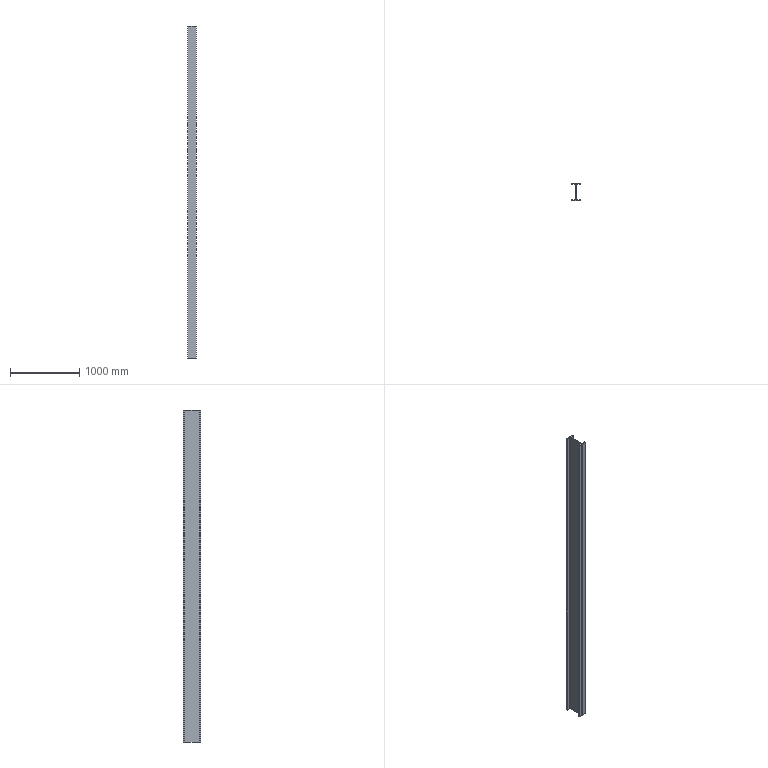Part | SolidWorks | features Extrusion 1 | 1 solid | 18 faces | box 125 x 250 x 4800 mm | volume 17745303 mm3 | plane 14 | cylinder 4 | commonest cylinder face diameters 16 x4
STEP:
#1=CARTESIAN_POINT('',(-62.5,9.,0.));
#2=VERTEX_POINT('',#1);
#3=CARTESIAN_POINT('',(-62.5,0.,0.));
#4=VERTEX_POINT('',#3);
#5=CARTESIAN_POINT('',(-62.5,0.,0.));
#6=DIRECTION('',(0.,-1.,0.));
#7=VECTOR('',#6,1000.);
#8=LINE('',#5,#7);
#9=EDGE_CURVE('',#2,#4,#8,.T.);
#10=ORIENTED_EDGE('',*,*,#9,.T.);
#11=CARTESIAN_POINT('',(-62.5,0.,4800.));
#12=VERTEX_POINT('',#11);
#13=CARTESIAN_POINT('',(-62.5,0.,4800.));
#14=DIRECTION('',(0.,0.,-1.));
#15=VECTOR('',#14,1000.);
#16=LINE('',#13,#15);
#17=EDGE_CURVE('',#12,#4,#16,.T.);
#18=ORIENTED_EDGE('',*,*,#17,.F.);
#19=CARTESIAN_POINT('',(-62.5,9.,4800.));
#20=VERTEX_POINT('',#19);
#21=CARTESIAN_POINT('',(-62.5,0.,4800.));
#22=DIRECTION('',(0.,-1.,0.));
#23=VECTOR('',#22,1000.);
#24=LINE('',#21,#23);
#25=EDGE_CURVE('',#20,#12,#24,.T.);
#26=ORIENTED_EDGE('',*,*,#25,.F.);
#27=CARTESIAN_POINT('',(-62.5,9.,4800.));
#28=DIRECTION('',(0.,0.,-1.));
#29=VECTOR('',#28,1000.);
#30=LINE('',#27,#29);
#31=EDGE_CURVE('',#20,#2,#30,.T.);
#32=ORIENTED_EDGE('',*,*,#31,.T.);
#33=EDGE_LOOP('',(#10,#18,#26,#32));
#34=FACE_OUTER_BOUND('',#33,.T.);
#35=CARTESIAN_POINT('',(-62.5,0.,4800.));
#36=DIRECTION('',(1.,0.,0.));
#37=DIRECTION('',(0.,0.,-1.));
#38=AXIS2_PLACEMENT_3D('',#35,#36,#37);
#39=PLANE('',#38);
#40=ADVANCED_FACE('',(#34),#39,.F.);
#41=CARTESIAN_POINT('',(62.5,0.,0.));
#42=VERTEX_POINT('',#41);
#43=CARTESIAN_POINT('',(62.5,0.,0.));
#44=DIRECTION('',(1.,0.,0.));
#45=VECTOR('',#44,1000.);
#46=LINE('',#43,#45);
#47=EDGE_CURVE('',#4,#42,#46,.T.);
#48=ORIENTED_EDGE('',*,*,#47,.T.);
#49=CARTESIAN_POINT('',(62.5,0.,4800.));
#50=VERTEX_POINT('',#49);
#51=CARTESIAN_POINT('',(62.5,0.,4800.));
#52=DIRECTION('',(0.,0.,-1.));
#53=VECTOR('',#52,1000.);
#54=LINE('',#51,#53);
#55=EDGE_CURVE('',#50,#42,#54,.T.);
#56=ORIENTED_EDGE('',*,*,#55,.F.);
#57=CARTESIAN_POINT('',(62.5,0.,4800.));
#58=DIRECTION('',(1.,0.,0.));
#59=VECTOR('',#58,1000.);
#60=LINE('',#57,#59);
#61=EDGE_CURVE('',#12,#50,#60,.T.);
#62=ORIENTED_EDGE('',*,*,#61,.F.);
#63=ORIENTED_EDGE('',*,*,#17,.T.);
#64=EDGE_LOOP('',(#48,#56,#62,#63));
#65=FACE_OUTER_BOUND('',#64,.T.);
#66=CARTESIAN_POINT('',(62.5,0.,4800.));
#67=DIRECTION('',(0.,1.,0.));
#68=DIRECTION('',(0.,0.,1.));
#69=AXIS2_PLACEMENT_3D('',#66,#67,#68);
#70=PLANE('',#69);
#71=ADVANCED_FACE('',(#65),#70,.F.);
#72=CARTESIAN_POINT('',(62.5,9.,0.));
#73=VERTEX_POINT('',#72);
#74=CARTESIAN_POINT('',(62.5,0.,0.));
#75=DIRECTION('',(0.,1.,0.));
#76=VECTOR('',#75,1000.);
#77=LINE('',#74,#76);
#78=EDGE_CURVE('',#42,#73,#77,.T.);
#79=ORIENTED_EDGE('',*,*,#78,.T.);
#80=CARTESIAN_POINT('',(62.5,9.,4800.));
#81=VERTEX_POINT('',#80);
#82=CARTESIAN_POINT('',(62.5,9.,4800.));
#83=DIRECTION('',(0.,0.,-1.));
#84=VECTOR('',#83,1000.);
#85=LINE('',#82,#84);
#86=EDGE_CURVE('',#81,#73,#85,.T.);
#87=ORIENTED_EDGE('',*,*,#86,.F.);
#88=CARTESIAN_POINT('',(62.5,0.,4800.));
#89=DIRECTION('',(0.,1.,0.));
#90=VECTOR('',#89,1000.);
#91=LINE('',#88,#90);
#92=EDGE_CURVE('',#50,#81,#91,.T.);
#93=ORIENTED_EDGE('',*,*,#92,.F.);
#94=ORIENTED_EDGE('',*,*,#55,.T.);
#95=EDGE_LOOP('',(#79,#87,#93,#94));
#96=FACE_OUTER_BOUND('',#95,.T.);
#97=CARTESIAN_POINT('',(62.5,0.,4800.));
#98=DIRECTION('',(-1.,0.,0.));
#99=DIRECTION('',(0.,0.,1.));
#100=AXIS2_PLACEMENT_3D('',#97,#98,#99);
#101=PLANE('',#100);
#102=ADVANCED_FACE('',(#96),#101,.F.);
#103=CARTESIAN_POINT('',(11.,9.,0.));
#104=VERTEX_POINT('',#103);
#105=CARTESIAN_POINT('',(62.5,9.,0.));
#106=DIRECTION('',(-1.,0.,0.));
#107=VECTOR('',#106,1000.);
#108=LINE('',#105,#107);
#109=EDGE_CURVE('',#73,#104,#108,.T.);
#110=ORIENTED_EDGE('',*,*,#109,.T.);
#111=CARTESIAN_POINT('',(11.,9.,4800.));
#112=VERTEX_POINT('',#111);
#113=CARTESIAN_POINT('',(11.,9.,4800.));
#114=DIRECTION('',(0.,0.,-1.));
#115=VECTOR('',#114,1000.);
#116=LINE('',#113,#115);
#117=EDGE_CURVE('',#112,#104,#116,.T.);
#118=ORIENTED_EDGE('',*,*,#117,.F.);
#119=CARTESIAN_POINT('',(62.5,9.,4800.));
#120=DIRECTION('',(-1.,0.,0.));
#121=VECTOR('',#120,1000.);
#122=LINE('',#119,#121);
#123=EDGE_CURVE('',#81,#112,#122,.T.);
#124=ORIENTED_EDGE('',*,*,#123,.F.);
#125=ORIENTED_EDGE('',*,*,#86,.T.);
#126=EDGE_LOOP('',(#110,#118,#124,#125));
#127=FACE_OUTER_BOUND('',#126,.T.);
#128=CARTESIAN_POINT('',(62.5,9.,4800.));
#129=DIRECTION('',(0.,-1.,0.));
#130=DIRECTION('',(0.,0.,-1.));
#131=AXIS2_PLACEMENT_3D('',#128,#129,#130);
#132=PLANE('',#131);
#133=ADVANCED_FACE('',(#127),#132,.F.);
#134=CARTESIAN_POINT('',(3.,17.,0.));
#135=VERTEX_POINT('',#134);
#136=CARTESIAN_POINT('',(11.,17.,0.));
#137=DIRECTION('',(0.,0.,-1.));
#138=DIRECTION('',(-1.,0.,0.));
#139=AXIS2_PLACEMENT_3D('',#136,#137,#138);
#140=CIRCLE('',#139,8.);
#141=EDGE_CURVE('',#104,#135,#140,.T.);
#142=ORIENTED_EDGE('',*,*,#141,.T.);
#143=CARTESIAN_POINT('',(3.,17.,4800.));
#144=VERTEX_POINT('',#143);
#145=CARTESIAN_POINT('',(3.,17.,4800.));
#146=DIRECTION('',(0.,0.,-1.));
#147=VECTOR('',#146,1000.);
#148=LINE('',#145,#147);
#149=EDGE_CURVE('',#144,#135,#148,.T.);
#150=ORIENTED_EDGE('',*,*,#149,.F.);
#151=CARTESIAN_POINT('',(11.,17.,4800.));
#152=DIRECTION('',(0.,0.,-1.));
#153=DIRECTION('',(-1.,0.,0.));
#154=AXIS2_PLACEMENT_3D('',#151,#152,#153);
#155=CIRCLE('',#154,8.);
#156=EDGE_CURVE('',#112,#144,#155,.T.);
#157=ORIENTED_EDGE('',*,*,#156,.F.);
#158=ORIENTED_EDGE('',*,*,#117,.T.);
#159=EDGE_LOOP('',(#142,#150,#157,#158));
#160=FACE_OUTER_BOUND('',#159,.T.);
#161=CARTESIAN_POINT('',(11.,17.,4800.));
#162=DIRECTION('',(0.,0.,-1.));
#163=DIRECTION('',(-1.,0.,0.));
#164=AXIS2_PLACEMENT_3D('',#161,#162,#163);
#165=CYLINDRICAL_SURFACE('',#164,8.);
#166=ADVANCED_FACE('',(#160),#165,.F.);
#167=CARTESIAN_POINT('',(3.,233.,0.));
#168=VERTEX_POINT('',#167);
#169=CARTESIAN_POINT('',(3.,17.,0.));
#170=DIRECTION('',(0.,1.,0.));
#171=VECTOR('',#170,1000.);
#172=LINE('',#169,#171);
#173=EDGE_CURVE('',#135,#168,#172,.T.);
#174=ORIENTED_EDGE('',*,*,#173,.T.);
#175=CARTESIAN_POINT('',(3.,233.,4800.));
#176=VERTEX_POINT('',#175);
#177=CARTESIAN_POINT('',(3.,233.,4800.));
#178=DIRECTION('',(0.,0.,-1.));
#179=VECTOR('',#178,1000.);
#180=LINE('',#177,#179);
#181=EDGE_CURVE('',#176,#168,#180,.T.);
#182=ORIENTED_EDGE('',*,*,#181,.F.);
#183=CARTESIAN_POINT('',(3.,17.,4800.));
#184=DIRECTION('',(0.,1.,0.));
#185=VECTOR('',#184,1000.);
#186=LINE('',#183,#185);
#187=EDGE_CURVE('',#144,#176,#186,.T.);
#188=ORIENTED_EDGE('',*,*,#187,.F.);
#189=ORIENTED_EDGE('',*,*,#149,.T.);
#190=EDGE_LOOP('',(#174,#182,#188,#189));
#191=FACE_OUTER_BOUND('',#190,.T.);
#192=CARTESIAN_POINT('',(3.,17.,4800.));
#193=DIRECTION('',(-1.,0.,0.));
#194=DIRECTION('',(0.,-1.,0.));
#195=AXIS2_PLACEMENT_3D('',#192,#193,#194);
#196=PLANE('',#195);
#197=ADVANCED_FACE('',(#191),#196,.F.);
#198=CARTESIAN_POINT('',(11.,241.,0.));
#199=VERTEX_POINT('',#198);
#200=CARTESIAN_POINT('',(11.,233.,0.));
#201=DIRECTION('',(0.,0.,-1.));
#202=DIRECTION('',(-1.,0.,0.));
#203=AXIS2_PLACEMENT_3D('',#200,#201,#202);
#204=CIRCLE('',#203,8.);
#205=EDGE_CURVE('',#168,#199,#204,.T.);
#206=ORIENTED_EDGE('',*,*,#205,.T.);
#207=CARTESIAN_POINT('',(11.,241.,4800.));
#208=VERTEX_POINT('',#207);
#209=CARTESIAN_POINT('',(11.,241.,4800.));
#210=DIRECTION('',(0.,0.,-1.));
#211=VECTOR('',#210,1000.);
#212=LINE('',#209,#211);
#213=EDGE_CURVE('',#208,#199,#212,.T.);
#214=ORIENTED_EDGE('',*,*,#213,.F.);
#215=CARTESIAN_POINT('',(11.,233.,4800.));
#216=DIRECTION('',(0.,0.,-1.));
#217=DIRECTION('',(-1.,0.,0.));
#218=AXIS2_PLACEMENT_3D('',#215,#216,#217);
#219=CIRCLE('',#218,8.);
#220=EDGE_CURVE('',#176,#208,#219,.T.);
#221=ORIENTED_EDGE('',*,*,#220,.F.);
#222=ORIENTED_EDGE('',*,*,#181,.T.);
#223=EDGE_LOOP('',(#206,#214,#221,#222));
#224=FACE_OUTER_BOUND('',#223,.T.);
#225=CARTESIAN_POINT('',(11.,233.,4800.));
#226=DIRECTION('',(0.,0.,-1.));
#227=DIRECTION('',(-1.,0.,0.));
#228=AXIS2_PLACEMENT_3D('',#225,#226,#227);
#229=CYLINDRICAL_SURFACE('',#228,8.);
#230=ADVANCED_FACE('',(#224),#229,.F.);
#231=CARTESIAN_POINT('',(62.5,241.,0.));
#232=VERTEX_POINT('',#231);
#233=CARTESIAN_POINT('',(11.,241.,0.));
#234=DIRECTION('',(1.,0.,0.));
#235=VECTOR('',#234,1000.);
#236=LINE('',#233,#235);
#237=EDGE_CURVE('',#199,#232,#236,.T.);
#238=ORIENTED_EDGE('',*,*,#237,.T.);
#239=CARTESIAN_POINT('',(62.5,241.,4800.));
#240=VERTEX_POINT('',#239);
#241=CARTESIAN_POINT('',(62.5,241.,4800.));
#242=DIRECTION('',(0.,0.,-1.));
#243=VECTOR('',#242,1000.);
#244=LINE('',#241,#243);
#245=EDGE_CURVE('',#240,#232,#244,.T.);
#246=ORIENTED_EDGE('',*,*,#245,.F.);
#247=CARTESIAN_POINT('',(11.,241.,4800.));
#248=DIRECTION('',(1.,0.,0.));
#249=VECTOR('',#248,1000.);
#250=LINE('',#247,#249);
#251=EDGE_CURVE('',#208,#240,#250,.T.);
#252=ORIENTED_EDGE('',*,*,#251,.F.);
#253=ORIENTED_EDGE('',*,*,#213,.T.);
#254=EDGE_LOOP('',(#238,#246,#252,#253));
#255=FACE_OUTER_BOUND('',#254,.T.);
#256=CARTESIAN_POINT('',(11.,241.,4800.));
#257=DIRECTION('',(0.,1.,0.));
#258=DIRECTION('',(0.,0.,1.));
#259=AXIS2_PLACEMENT_3D('',#256,#257,#258);
#260=PLANE('',#259);
#261=ADVANCED_FACE('',(#255),#260,.F.);
#262=CARTESIAN_POINT('',(62.5,250.,0.));
#263=VERTEX_POINT('',#262);
#264=CARTESIAN_POINT('',(62.5,241.,0.));
#265=DIRECTION('',(0.,1.,0.));
#266=VECTOR('',#265,1000.);
#267=LINE('',#264,#266);
#268=EDGE_CURVE('',#232,#263,#267,.T.);
#269=ORIENTED_EDGE('',*,*,#268,.T.);
#270=CARTESIAN_POINT('',(62.5,250.,4800.));
#271=VERTEX_POINT('',#270);
#272=CARTESIAN_POINT('',(62.5,250.,4800.));
#273=DIRECTION('',(0.,0.,-1.));
#274=VECTOR('',#273,1000.);
#275=LINE('',#272,#274);
#276=EDGE_CURVE('',#271,#263,#275,.T.);
#277=ORIENTED_EDGE('',*,*,#276,.F.);
#278=CARTESIAN_POINT('',(62.5,241.,4800.));
#279=DIRECTION('',(0.,1.,0.));
#280=VECTOR('',#279,1000.);
#281=LINE('',#278,#280);
#282=EDGE_CURVE('',#240,#271,#281,.T.);
#283=ORIENTED_EDGE('',*,*,#282,.F.);
#284=ORIENTED_EDGE('',*,*,#245,.T.);
#285=EDGE_LOOP('',(#269,#277,#283,#284));
#286=FACE_OUTER_BOUND('',#285,.T.);
#287=CARTESIAN_POINT('',(62.5,241.,4800.));
#288=DIRECTION('',(-1.,0.,0.));
#289=DIRECTION('',(0.,0.,1.));
#290=AXIS2_PLACEMENT_3D('',#287,#288,#289);
#291=PLANE('',#290);
#292=ADVANCED_FACE('',(#286),#291,.F.);
#293=CARTESIAN_POINT('',(-62.5,250.,0.));
#294=VERTEX_POINT('',#293);
#295=CARTESIAN_POINT('',(-62.5,250.,0.));
#296=DIRECTION('',(-1.,0.,0.));
#297=VECTOR('',#296,1000.);
#298=LINE('',#295,#297);
#299=EDGE_CURVE('',#263,#294,#298,.T.);
#300=ORIENTED_EDGE('',*,*,#299,.T.);
#301=CARTESIAN_POINT('',(-62.5,250.,4800.));
#302=VERTEX_POINT('',#301);
#303=CARTESIAN_POINT('',(-62.5,250.,4800.));
#304=DIRECTION('',(0.,0.,-1.));
#305=VECTOR('',#304,1000.);
#306=LINE('',#303,#305);
#307=EDGE_CURVE('',#302,#294,#306,.T.);
#308=ORIENTED_EDGE('',*,*,#307,.F.);
#309=CARTESIAN_POINT('',(-62.5,250.,4800.));
#310=DIRECTION('',(-1.,0.,0.));
#311=VECTOR('',#310,1000.);
#312=LINE('',#309,#311);
#313=EDGE_CURVE('',#271,#302,#312,.T.);
#314=ORIENTED_EDGE('',*,*,#313,.F.);
#315=ORIENTED_EDGE('',*,*,#276,.T.);
#316=EDGE_LOOP('',(#300,#308,#314,#315));
#317=FACE_OUTER_BOUND('',#316,.T.);
#318=CARTESIAN_POINT('',(-62.5,250.,4800.));
#319=DIRECTION('',(0.,-1.,0.));
#320=DIRECTION('',(1.,0.,0.));
#321=AXIS2_PLACEMENT_3D('',#318,#319,#320);
#322=PLANE('',#321);
#323=ADVANCED_FACE('',(#317),#322,.F.);
#324=CARTESIAN_POINT('',(-62.5,241.,0.));
#325=VERTEX_POINT('',#324);
#326=CARTESIAN_POINT('',(-62.5,241.,0.));
#327=DIRECTION('',(0.,-1.,0.));
#328=VECTOR('',#327,1000.);
#329=LINE('',#326,#328);
#330=EDGE_CURVE('',#294,#325,#329,.T.);
#331=ORIENTED_EDGE('',*,*,#330,.T.);
#332=CARTESIAN_POINT('',(-62.5,241.,4800.));
#333=VERTEX_POINT('',#332);
#334=CARTESIAN_POINT('',(-62.5,241.,4800.));
#335=DIRECTION('',(0.,0.,-1.));
#336=VECTOR('',#335,1000.);
#337=LINE('',#334,#336);
#338=EDGE_CURVE('',#333,#325,#337,.T.);
#339=ORIENTED_EDGE('',*,*,#338,.F.);
#340=CARTESIAN_POINT('',(-62.5,241.,4800.));
#341=DIRECTION('',(0.,-1.,0.));
#342=VECTOR('',#341,1000.);
#343=LINE('',#340,#342);
#344=EDGE_CURVE('',#302,#333,#343,.T.);
#345=ORIENTED_EDGE('',*,*,#344,.F.);
#346=ORIENTED_EDGE('',*,*,#307,.T.);
#347=EDGE_LOOP('',(#331,#339,#345,#346));
#348=FACE_OUTER_BOUND('',#347,.T.);
#349=CARTESIAN_POINT('',(-62.5,241.,4800.));
#350=DIRECTION('',(1.,0.,0.));
#351=DIRECTION('',(0.,0.,-1.));
#352=AXIS2_PLACEMENT_3D('',#349,#350,#351);
#353=PLANE('',#352);
#354=ADVANCED_FACE('',(#348),#353,.F.);
#355=CARTESIAN_POINT('',(-11.,241.,0.));
#356=VERTEX_POINT('',#355);
#357=CARTESIAN_POINT('',(-11.,241.,0.));
#358=DIRECTION('',(1.,0.,0.));
#359=VECTOR('',#358,1000.);
#360=LINE('',#357,#359);
#361=EDGE_CURVE('',#325,#356,#360,.T.);
#362=ORIENTED_EDGE('',*,*,#361,.T.);
#363=CARTESIAN_POINT('',(-11.,241.,4800.));
#364=VERTEX_POINT('',#363);
#365=CARTESIAN_POINT('',(-11.,241.,4800.));
#366=DIRECTION('',(0.,0.,-1.));
#367=VECTOR('',#366,1000.);
#368=LINE('',#365,#367);
#369=EDGE_CURVE('',#364,#356,#368,.T.);
#370=ORIENTED_EDGE('',*,*,#369,.F.);
#371=CARTESIAN_POINT('',(-11.,241.,4800.));
#372=DIRECTION('',(1.,0.,0.));
#373=VECTOR('',#372,1000.);
#374=LINE('',#371,#373);
#375=EDGE_CURVE('',#333,#364,#374,.T.);
#376=ORIENTED_EDGE('',*,*,#375,.F.);
#377=ORIENTED_EDGE('',*,*,#338,.T.);
#378=EDGE_LOOP('',(#362,#370,#376,#377));
#379=FACE_OUTER_BOUND('',#378,.T.);
#380=CARTESIAN_POINT('',(-11.,241.,4800.));
#381=DIRECTION('',(0.,1.,0.));
#382=DIRECTION('',(0.,0.,1.));
#383=AXIS2_PLACEMENT_3D('',#380,#381,#382);
#384=PLANE('',#383);
#385=ADVANCED_FACE('',(#379),#384,.F.);
#386=CARTESIAN_POINT('',(-3.,233.,0.));
#387=VERTEX_POINT('',#386);
#388=CARTESIAN_POINT('',(-11.,233.,0.));
#389=DIRECTION('',(0.,0.,-1.));
#390=DIRECTION('',(1.,0.,0.));
#391=AXIS2_PLACEMENT_3D('',#388,#389,#390);
#392=CIRCLE('',#391,8.);
#393=EDGE_CURVE('',#356,#387,#392,.T.);
#394=ORIENTED_EDGE('',*,*,#393,.T.);
#395=CARTESIAN_POINT('',(-3.,233.,4800.));
#396=VERTEX_POINT('',#395);
#397=CARTESIAN_POINT('',(-3.,233.,4800.));
#398=DIRECTION('',(0.,0.,-1.));
#399=VECTOR('',#398,1000.);
#400=LINE('',#397,#399);
#401=EDGE_CURVE('',#396,#387,#400,.T.);
#402=ORIENTED_EDGE('',*,*,#401,.F.);
#403=CARTESIAN_POINT('',(-11.,233.,4800.));
#404=DIRECTION('',(0.,0.,-1.));
#405=DIRECTION('',(1.,0.,0.));
#406=AXIS2_PLACEMENT_3D('',#403,#404,#405);
#407=CIRCLE('',#406,8.);
#408=EDGE_CURVE('',#364,#396,#407,.T.);
#409=ORIENTED_EDGE('',*,*,#408,.F.);
#410=ORIENTED_EDGE('',*,*,#369,.T.);
#411=EDGE_LOOP('',(#394,#402,#409,#410));
#412=FACE_OUTER_BOUND('',#411,.T.);
#413=CARTESIAN_POINT('',(-11.,233.,4800.));
#414=DIRECTION('',(0.,0.,-1.));
#415=DIRECTION('',(-1.,0.,0.));
#416=AXIS2_PLACEMENT_3D('',#413,#414,#415);
#417=CYLINDRICAL_SURFACE('',#416,8.);
#418=ADVANCED_FACE('',(#412),#417,.F.);
#419=CARTESIAN_POINT('',(-3.,17.,0.));
#420=VERTEX_POINT('',#419);
#421=CARTESIAN_POINT('',(-3.,17.,0.));
#422=DIRECTION('',(0.,-1.,0.));
#423=VECTOR('',#422,1000.);
#424=LINE('',#421,#423);
#425=EDGE_CURVE('',#387,#420,#424,.T.);
#426=ORIENTED_EDGE('',*,*,#425,.T.);
#427=CARTESIAN_POINT('',(-3.,17.,4800.));
#428=VERTEX_POINT('',#427);
#429=CARTESIAN_POINT('',(-3.,17.,4800.));
#430=DIRECTION('',(0.,0.,-1.));
#431=VECTOR('',#430,1000.);
#432=LINE('',#429,#431);
#433=EDGE_CURVE('',#428,#420,#432,.T.);
#434=ORIENTED_EDGE('',*,*,#433,.F.);
#435=CARTESIAN_POINT('',(-3.,17.,4800.));
#436=DIRECTION('',(0.,-1.,0.));
#437=VECTOR('',#436,1000.);
#438=LINE('',#435,#437);
#439=EDGE_CURVE('',#396,#428,#438,.T.);
#440=ORIENTED_EDGE('',*,*,#439,.F.);
#441=ORIENTED_EDGE('',*,*,#401,.T.);
#442=EDGE_LOOP('',(#426,#434,#440,#441));
#443=FACE_OUTER_BOUND('',#442,.T.);
#444=CARTESIAN_POINT('',(-3.,17.,4800.));
#445=DIRECTION('',(1.,0.,0.));
#446=DIRECTION('',(0.,1.,0.));
#447=AXIS2_PLACEMENT_3D('',#444,#445,#446);
#448=PLANE('',#447);
#449=ADVANCED_FACE('',(#443),#448,.F.);
#450=CARTESIAN_POINT('',(-11.,9.,0.));
#451=VERTEX_POINT('',#450);
#452=CARTESIAN_POINT('',(-11.,17.,0.));
#453=DIRECTION('',(0.,0.,-1.));
#454=DIRECTION('',(-1.,0.,0.));
#455=AXIS2_PLACEMENT_3D('',#452,#453,#454);
#456=CIRCLE('',#455,8.);
#457=EDGE_CURVE('',#420,#451,#456,.T.);
#458=ORIENTED_EDGE('',*,*,#457,.T.);
#459=CARTESIAN_POINT('',(-11.,9.,4800.));
#460=VERTEX_POINT('',#459);
#461=CARTESIAN_POINT('',(-11.,9.,4800.));
#462=DIRECTION('',(0.,0.,-1.));
#463=VECTOR('',#462,1000.);
#464=LINE('',#461,#463);
#465=EDGE_CURVE('',#460,#451,#464,.T.);
#466=ORIENTED_EDGE('',*,*,#465,.F.);
#467=CARTESIAN_POINT('',(-11.,17.,4800.));
#468=DIRECTION('',(0.,0.,-1.));
#469=DIRECTION('',(-1.,0.,0.));
#470=AXIS2_PLACEMENT_3D('',#467,#468,#469);
#471=CIRCLE('',#470,8.);
#472=EDGE_CURVE('',#428,#460,#471,.T.);
#473=ORIENTED_EDGE('',*,*,#472,.F.);
#474=ORIENTED_EDGE('',*,*,#433,.T.);
#475=EDGE_LOOP('',(#458,#466,#473,#474));
#476=FACE_OUTER_BOUND('',#475,.T.);
#477=CARTESIAN_POINT('',(-11.,17.,4800.));
#478=DIRECTION('',(0.,0.,-1.));
#479=DIRECTION('',(-1.,0.,0.));
#480=AXIS2_PLACEMENT_3D('',#477,#478,#479);
#481=CYLINDRICAL_SURFACE('',#480,8.);
#482=ADVANCED_FACE('',(#476),#481,.F.);
#483=CARTESIAN_POINT('',(-62.5,9.,0.));
#484=DIRECTION('',(-1.,0.,0.));
#485=VECTOR('',#484,1000.);
#486=LINE('',#483,#485);
#487=EDGE_CURVE('',#451,#2,#486,.T.);
#488=ORIENTED_EDGE('',*,*,#487,.T.);
#489=ORIENTED_EDGE('',*,*,#31,.F.);
#490=CARTESIAN_POINT('',(-62.5,9.,4800.));
#491=DIRECTION('',(-1.,0.,0.));
#492=VECTOR('',#491,1000.);
#493=LINE('',#490,#492);
#494=EDGE_CURVE('',#460,#20,#493,.T.);
#495=ORIENTED_EDGE('',*,*,#494,.F.);
#496=ORIENTED_EDGE('',*,*,#465,.T.);
#497=EDGE_LOOP('',(#488,#489,#495,#496));
#498=FACE_OUTER_BOUND('',#497,.T.);
#499=CARTESIAN_POINT('',(-62.5,9.,4800.));
#500=DIRECTION('',(0.,-1.,0.));
#501=DIRECTION('',(0.,0.,-1.));
#502=AXIS2_PLACEMENT_3D('',#499,#500,#501);
#503=PLANE('',#502);
#504=ADVANCED_FACE('',(#498),#503,.F.);
#505=ORIENTED_EDGE('',*,*,#25,.T.);
#506=ORIENTED_EDGE('',*,*,#61,.T.);
#507=ORIENTED_EDGE('',*,*,#92,.T.);
#508=ORIENTED_EDGE('',*,*,#123,.T.);
#509=ORIENTED_EDGE('',*,*,#156,.T.);
#510=ORIENTED_EDGE('',*,*,#187,.T.);
#511=ORIENTED_EDGE('',*,*,#220,.T.);
#512=ORIENTED_EDGE('',*,*,#251,.T.);
#513=ORIENTED_EDGE('',*,*,#282,.T.);
#514=ORIENTED_EDGE('',*,*,#313,.T.);
#515=ORIENTED_EDGE('',*,*,#344,.T.);
#516=ORIENTED_EDGE('',*,*,#375,.T.);
#517=ORIENTED_EDGE('',*,*,#408,.T.);
#518=ORIENTED_EDGE('',*,*,#439,.T.);
#519=ORIENTED_EDGE('',*,*,#472,.T.);
#520=ORIENTED_EDGE('',*,*,#494,.T.);
#521=EDGE_LOOP('',(#505,#506,#507,#508,#509,#510,#511,#512,#513,#514,#515,#516,#517,#518,#519,#520));
#522=FACE_OUTER_BOUND('',#521,.T.);
#523=CARTESIAN_POINT('',(-11.,17.,4800.));
#524=DIRECTION('',(0.,0.,-1.));
#525=DIRECTION('',(-1.,0.,0.));
#526=AXIS2_PLACEMENT_3D('',#523,#524,#525);
#527=PLANE('',#526);
#528=ADVANCED_FACE('',(#522),#527,.F.);
#529=ORIENTED_EDGE('',*,*,#9,.F.);
#530=ORIENTED_EDGE('',*,*,#487,.F.);
#531=ORIENTED_EDGE('',*,*,#457,.F.);
#532=ORIENTED_EDGE('',*,*,#425,.F.);
#533=ORIENTED_EDGE('',*,*,#393,.F.);
#534=ORIENTED_EDGE('',*,*,#361,.F.);
#535=ORIENTED_EDGE('',*,*,#330,.F.);
#536=ORIENTED_EDGE('',*,*,#299,.F.);
#537=ORIENTED_EDGE('',*,*,#268,.F.);
#538=ORIENTED_EDGE('',*,*,#237,.F.);
#539=ORIENTED_EDGE('',*,*,#205,.F.);
#540=ORIENTED_EDGE('',*,*,#173,.F.);
#541=ORIENTED_EDGE('',*,*,#141,.F.);
#542=ORIENTED_EDGE('',*,*,#109,.F.);
#543=ORIENTED_EDGE('',*,*,#78,.F.);
#544=ORIENTED_EDGE('',*,*,#47,.F.);
#545=EDGE_LOOP('',(#529,#530,#531,#532,#533,#534,#535,#536,#537,#538,#539,#540,#541,#542,#543,#544));
#546=FACE_OUTER_BOUND('',#545,.T.);
#547=CARTESIAN_POINT('',(-11.,17.,0.));
#548=DIRECTION('',(0.,0.,-1.));
#549=DIRECTION('',(-1.,0.,0.));
#550=AXIS2_PLACEMENT_3D('',#547,#548,#549);
#551=PLANE('',#550);
#552=ADVANCED_FACE('',(#546),#551,.T.);
#553=CLOSED_SHELL('',(#40,#71,#102,#133,#166,#197,#230,#261,#292,#323,#354,#385,#418,#449,#482,#504,#528,#552));
#554=MANIFOLD_SOLID_BREP('',#553);
#555=CARTESIAN_POINT('',(0.,0.,0.));
#556=DIRECTION('',(0.,0.,1.));
#557=DIRECTION('',(1.,0.,0.));
#558=AXIS2_PLACEMENT_3D('',#555,#556,#557);
#559=(LENGTH_UNIT()NAMED_UNIT(*)SI_UNIT(.MILLI.,.METRE.));
#560=UNCERTAINTY_MEASURE_WITH_UNIT(LENGTH_MEASURE(0.00001),#559,'','');
#561=(NAMED_UNIT(*)PLANE_ANGLE_UNIT()SI_UNIT($,.RADIAN.));
#562=(NAMED_UNIT(*)SI_UNIT($,.STERADIAN.)SOLID_ANGLE_UNIT());
#563=(GEOMETRIC_REPRESENTATION_CONTEXT(3)GLOBAL_UNCERTAINTY_ASSIGNED_CONTEXT((#560))GLOBAL_UNIT_ASSIGNED_CONTEXT((#559,#561,#562))REPRESENTATION_CONTEXT('',''));
#564=ADVANCED_BREP_SHAPE_REPRESENTATION('',(#554,#558),#563);